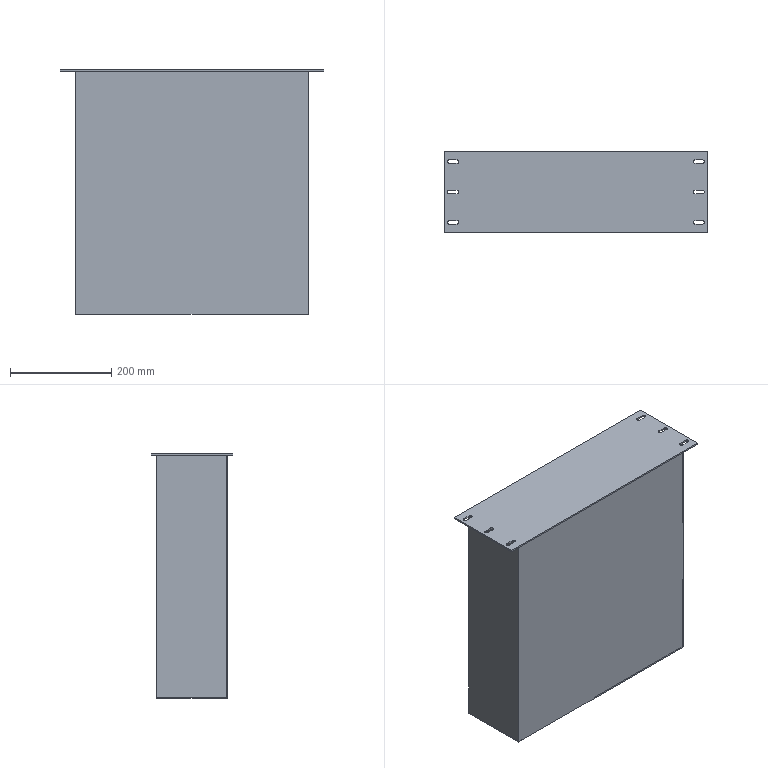Part | STEP file | FCT electrical control box | 1 solid | 45 faces | box 520 x 160 x 483 mm | volume 872599 mm3 | plane 27 | cylinder 18 | commonest cylinder face diameters 7 x18